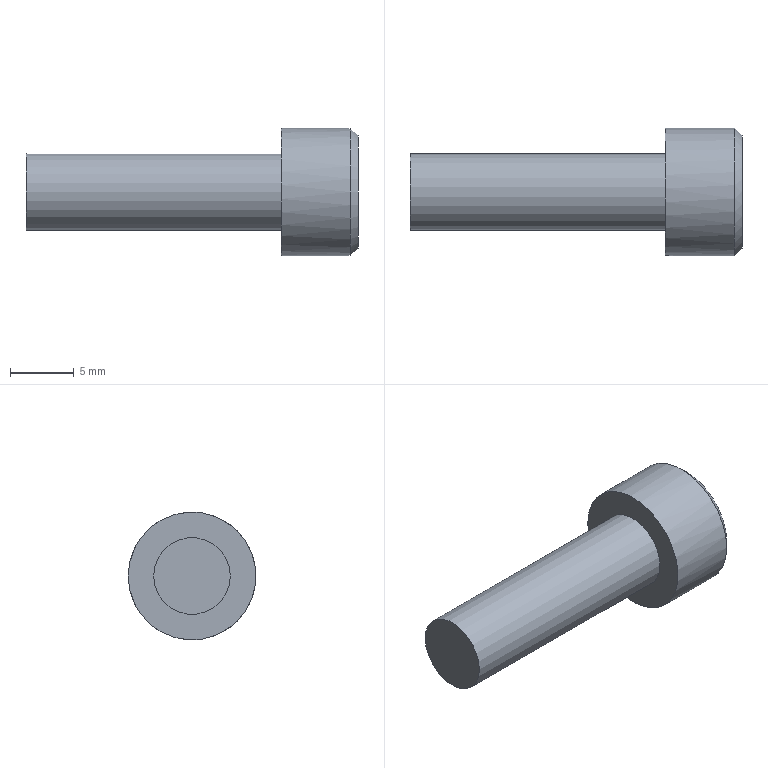Part | NX | features 5003_310_CB6-20 2 | 1 solid | 19 faces | box 26 x 10 x 10 mm | volume 956.513 mm3 | plane 15 | cylinder 2 | cone 2 | commonest cylinder face diameters 6 x1 10 x1
STEP:
#1=CARTESIAN_POINT('',(309.625,-201.4,-97.));
#2=VERTEX_POINT('',#1);
#3=CARTESIAN_POINT('',(309.625,-197.,-97.));
#4=DIRECTION('',(-1.,0.,0.));
#5=DIRECTION('',(0.,-1.,0.));
#6=AXIS2_PLACEMENT_3D('',#3,#4,#5);
#7=CIRCLE('',#6,4.4);
#8=EDGE_CURVE('',#2,#2,#7,.F.);
#9=ORIENTED_EDGE('',*,*,#8,.T.);
#10=EDGE_LOOP('',(#9));
#11=FACE_BOUND('',#10,.T.);
#12=CARTESIAN_POINT('',(309.625,-197.,-99.887));
#13=VERTEX_POINT('',#12);
#14=CARTESIAN_POINT('',(309.625,-194.5,-98.443));
#15=VERTEX_POINT('',#14);
#16=CARTESIAN_POINT('',(309.625,-197.,-99.887));
#17=DIRECTION('',(0.,0.866,0.5));
#18=VECTOR('',#17,1000.);
#19=LINE('',#16,#18);
#20=EDGE_CURVE('',#13,#15,#19,.T.);
#21=ORIENTED_EDGE('',*,*,#20,.F.);
#22=CARTESIAN_POINT('',(309.625,-199.5,-98.443));
#23=VERTEX_POINT('',#22);
#24=CARTESIAN_POINT('',(309.625,-199.5,-98.443));
#25=DIRECTION('',(0.,0.866,-0.5));
#26=VECTOR('',#25,1000.);
#27=LINE('',#24,#26);
#28=EDGE_CURVE('',#23,#13,#27,.T.);
#29=ORIENTED_EDGE('',*,*,#28,.F.);
#30=CARTESIAN_POINT('',(309.625,-199.5,-95.557));
#31=VERTEX_POINT('',#30);
#32=CARTESIAN_POINT('',(309.625,-199.5,-95.557));
#33=DIRECTION('',(0.,0.,-1.));
#34=VECTOR('',#33,1000.);
#35=LINE('',#32,#34);
#36=EDGE_CURVE('',#31,#23,#35,.T.);
#37=ORIENTED_EDGE('',*,*,#36,.F.);
#38=CARTESIAN_POINT('',(309.625,-197.,-94.113));
#39=VERTEX_POINT('',#38);
#40=CARTESIAN_POINT('',(309.625,-197.,-94.113));
#41=DIRECTION('',(0.,-0.866,-0.5));
#42=VECTOR('',#41,1000.);
#43=LINE('',#40,#42);
#44=EDGE_CURVE('',#39,#31,#43,.T.);
#45=ORIENTED_EDGE('',*,*,#44,.F.);
#46=CARTESIAN_POINT('',(309.625,-194.5,-95.557));
#47=VERTEX_POINT('',#46);
#48=CARTESIAN_POINT('',(309.625,-194.5,-95.557));
#49=DIRECTION('',(0.,-0.866,0.5));
#50=VECTOR('',#49,1000.);
#51=LINE('',#48,#50);
#52=EDGE_CURVE('',#47,#39,#51,.T.);
#53=ORIENTED_EDGE('',*,*,#52,.F.);
#54=CARTESIAN_POINT('',(309.625,-194.5,-98.443));
#55=DIRECTION('',(0.,0.,1.));
#56=VECTOR('',#55,1000.);
#57=LINE('',#54,#56);
#58=EDGE_CURVE('',#15,#47,#57,.T.);
#59=ORIENTED_EDGE('',*,*,#58,.F.);
#60=EDGE_LOOP('',(#21,#29,#37,#45,#53,#59));
#61=FACE_BOUND('',#60,.T.);
#62=CARTESIAN_POINT('',(309.625,-197.,-92.));
#63=DIRECTION('',(-1.,0.,0.));
#64=DIRECTION('',(0.,-1.,0.));
#65=AXIS2_PLACEMENT_3D('',#62,#63,#64);
#66=PLANE('',#65);
#67=ADVANCED_FACE('',(#11,#61),#66,.F.);
#68=CARTESIAN_POINT('',(283.625,-194.,-97.));
#69=VERTEX_POINT('',#68);
#70=CARTESIAN_POINT('',(283.625,-197.,-97.));
#71=DIRECTION('',(1.,0.,0.));
#72=DIRECTION('',(0.,1.,0.));
#73=AXIS2_PLACEMENT_3D('',#70,#71,#72);
#74=CIRCLE('',#73,3.);
#75=EDGE_CURVE('',#69,#69,#74,.T.);
#76=ORIENTED_EDGE('',*,*,#75,.F.);
#77=EDGE_LOOP('',(#76));
#78=FACE_BOUND('',#77,.T.);
#79=CARTESIAN_POINT('',(283.625,-197.,-97.));
#80=DIRECTION('',(1.,0.,0.));
#81=DIRECTION('',(0.,1.,0.));
#82=AXIS2_PLACEMENT_3D('',#79,#80,#81);
#83=PLANE('',#82);
#84=ADVANCED_FACE('',(#78),#83,.F.);
#85=CARTESIAN_POINT('',(303.625,-194.,-97.));
#86=VERTEX_POINT('',#85);
#87=CARTESIAN_POINT('',(303.625,-197.,-97.));
#88=DIRECTION('',(1.,0.,0.));
#89=DIRECTION('',(0.,1.,0.));
#90=AXIS2_PLACEMENT_3D('',#87,#88,#89);
#91=CIRCLE('',#90,3.);
#92=EDGE_CURVE('',#86,#86,#91,.T.);
#93=ORIENTED_EDGE('',*,*,#92,.F.);
#94=EDGE_LOOP('',(#93));
#95=FACE_BOUND('',#94,.T.);
#96=ORIENTED_EDGE('',*,*,#75,.T.);
#97=EDGE_LOOP('',(#96));
#98=FACE_BOUND('',#97,.T.);
#99=CARTESIAN_POINT('',(309.625,-197.,-97.));
#100=DIRECTION('',(1.,0.,0.));
#101=DIRECTION('',(0.,1.,0.));
#102=AXIS2_PLACEMENT_3D('',#99,#100,#101);
#103=CYLINDRICAL_SURFACE('',#102,3.);
#104=ADVANCED_FACE('',(#95,#98),#103,.T.);
#105=CARTESIAN_POINT('',(303.625,-192.,-97.));
#106=VERTEX_POINT('',#105);
#107=CARTESIAN_POINT('',(303.625,-197.,-97.));
#108=DIRECTION('',(1.,0.,0.));
#109=DIRECTION('',(0.,1.,0.));
#110=AXIS2_PLACEMENT_3D('',#107,#108,#109);
#111=CIRCLE('',#110,5.);
#112=EDGE_CURVE('',#106,#106,#111,.T.);
#113=ORIENTED_EDGE('',*,*,#112,.F.);
#114=EDGE_LOOP('',(#113));
#115=FACE_BOUND('',#114,.T.);
#116=ORIENTED_EDGE('',*,*,#92,.T.);
#117=EDGE_LOOP('',(#116));
#118=FACE_BOUND('',#117,.T.);
#119=CARTESIAN_POINT('',(303.625,-197.,-94.));
#120=DIRECTION('',(1.,0.,0.));
#121=DIRECTION('',(0.,1.,0.));
#122=AXIS2_PLACEMENT_3D('',#119,#120,#121);
#123=PLANE('',#122);
#124=ADVANCED_FACE('',(#115,#118),#123,.F.);
#125=CARTESIAN_POINT('',(309.025,-202.,-97.));
#126=VERTEX_POINT('',#125);
#127=CARTESIAN_POINT('',(309.025,-197.,-97.));
#128=DIRECTION('',(-1.,0.,0.));
#129=DIRECTION('',(0.,-1.,0.));
#130=AXIS2_PLACEMENT_3D('',#127,#128,#129);
#131=CIRCLE('',#130,5.);
#132=EDGE_CURVE('',#126,#126,#131,.T.);
#133=ORIENTED_EDGE('',*,*,#132,.T.);
#134=EDGE_LOOP('',(#133));
#135=FACE_BOUND('',#134,.T.);
#136=ORIENTED_EDGE('',*,*,#112,.T.);
#137=EDGE_LOOP('',(#136));
#138=FACE_BOUND('',#137,.T.);
#139=CARTESIAN_POINT('',(309.625,-197.,-97.));
#140=DIRECTION('',(1.,0.,0.));
#141=DIRECTION('',(0.,1.,0.));
#142=AXIS2_PLACEMENT_3D('',#139,#140,#141);
#143=CYLINDRICAL_SURFACE('',#142,5.);
#144=ADVANCED_FACE('',(#135,#138),#143,.T.);
#145=ORIENTED_EDGE('',*,*,#132,.F.);
#146=EDGE_LOOP('',(#145));
#147=FACE_BOUND('',#146,.T.);
#148=ORIENTED_EDGE('',*,*,#8,.F.);
#149=EDGE_LOOP('',(#148));
#150=FACE_BOUND('',#149,.T.);
#151=CARTESIAN_POINT('',(309.625,-197.,-97.));
#152=DIRECTION('',(-1.,0.,0.));
#153=DIRECTION('',(0.,-1.,0.));
#154=AXIS2_PLACEMENT_3D('',#151,#152,#153);
#155=CONICAL_SURFACE('',#154,4.4,0.7854);
#156=ADVANCED_FACE('',(#147,#150),#155,.T.);
#157=CARTESIAN_POINT('',(306.625,-199.5,-98.443));
#158=VERTEX_POINT('',#157);
#159=CARTESIAN_POINT('',(306.625,-198.25,-99.165));
#160=VERTEX_POINT('',#159);
#161=CARTESIAN_POINT('',(306.625,-199.5,-98.443));
#162=DIRECTION('',(0.,0.866,-0.5));
#163=VECTOR('',#162,1000.);
#164=LINE('',#161,#163);
#165=EDGE_CURVE('',#158,#160,#164,.T.);
#166=ORIENTED_EDGE('',*,*,#165,.F.);
#167=CARTESIAN_POINT('',(306.625,-199.5,-98.443));
#168=DIRECTION('',(1.,0.,0.));
#169=VECTOR('',#168,1000.);
#170=LINE('',#167,#169);
#171=EDGE_CURVE('',#158,#23,#170,.T.);
#172=ORIENTED_EDGE('',*,*,#171,.T.);
#173=ORIENTED_EDGE('',*,*,#28,.T.);
#174=CARTESIAN_POINT('',(306.625,-197.,-99.887));
#175=VERTEX_POINT('',#174);
#176=CARTESIAN_POINT('',(306.625,-197.,-99.887));
#177=DIRECTION('',(1.,0.,0.));
#178=VECTOR('',#177,1000.);
#179=LINE('',#176,#178);
#180=EDGE_CURVE('',#175,#13,#179,.T.);
#181=ORIENTED_EDGE('',*,*,#180,.F.);
#182=CARTESIAN_POINT('',(306.625,-199.5,-98.443));
#183=DIRECTION('',(0.,0.866,-0.5));
#184=VECTOR('',#183,1000.);
#185=LINE('',#182,#184);
#186=EDGE_CURVE('',#160,#175,#185,.T.);
#187=ORIENTED_EDGE('',*,*,#186,.F.);
#188=EDGE_LOOP('',(#166,#172,#173,#181,#187));
#189=FACE_BOUND('',#188,.T.);
#190=CARTESIAN_POINT('',(306.625,-199.5,-98.443));
#191=DIRECTION('',(0.,-0.5,-0.866));
#192=DIRECTION('',(0.,-0.866,0.5));
#193=AXIS2_PLACEMENT_3D('',#190,#191,#192);
#194=PLANE('',#193);
#195=ADVANCED_FACE('',(#189),#194,.F.);
#196=CARTESIAN_POINT('',(306.625,-199.5,-95.557));
#197=VERTEX_POINT('',#196);
#198=CARTESIAN_POINT('',(306.625,-199.5,-97.));
#199=VERTEX_POINT('',#198);
#200=CARTESIAN_POINT('',(306.625,-199.5,-95.557));
#201=DIRECTION('',(0.,0.,-1.));
#202=VECTOR('',#201,1000.);
#203=LINE('',#200,#202);
#204=EDGE_CURVE('',#197,#199,#203,.T.);
#205=ORIENTED_EDGE('',*,*,#204,.F.);
#206=CARTESIAN_POINT('',(306.625,-199.5,-95.557));
#207=DIRECTION('',(1.,0.,0.));
#208=VECTOR('',#207,1000.);
#209=LINE('',#206,#208);
#210=EDGE_CURVE('',#197,#31,#209,.T.);
#211=ORIENTED_EDGE('',*,*,#210,.T.);
#212=ORIENTED_EDGE('',*,*,#36,.T.);
#213=ORIENTED_EDGE('',*,*,#171,.F.);
#214=CARTESIAN_POINT('',(306.625,-199.5,-95.557));
#215=DIRECTION('',(0.,0.,-1.));
#216=VECTOR('',#215,1000.);
#217=LINE('',#214,#216);
#218=EDGE_CURVE('',#199,#158,#217,.T.);
#219=ORIENTED_EDGE('',*,*,#218,.F.);
#220=EDGE_LOOP('',(#205,#211,#212,#213,#219));
#221=FACE_BOUND('',#220,.T.);
#222=CARTESIAN_POINT('',(306.625,-199.5,-95.557));
#223=DIRECTION('',(0.,-1.,0.));
#224=DIRECTION('',(0.,0.,1.));
#225=AXIS2_PLACEMENT_3D('',#222,#223,#224);
#226=PLANE('',#225);
#227=ADVANCED_FACE('',(#221),#226,.F.);
#228=CARTESIAN_POINT('',(306.625,-197.,-94.113));
#229=VERTEX_POINT('',#228);
#230=CARTESIAN_POINT('',(306.625,-198.25,-94.835));
#231=VERTEX_POINT('',#230);
#232=CARTESIAN_POINT('',(306.625,-197.,-94.113));
#233=DIRECTION('',(0.,-0.866,-0.5));
#234=VECTOR('',#233,1000.);
#235=LINE('',#232,#234);
#236=EDGE_CURVE('',#229,#231,#235,.T.);
#237=ORIENTED_EDGE('',*,*,#236,.F.);
#238=CARTESIAN_POINT('',(306.625,-197.,-94.113));
#239=DIRECTION('',(1.,0.,0.));
#240=VECTOR('',#239,1000.);
#241=LINE('',#238,#240);
#242=EDGE_CURVE('',#229,#39,#241,.T.);
#243=ORIENTED_EDGE('',*,*,#242,.T.);
#244=ORIENTED_EDGE('',*,*,#44,.T.);
#245=ORIENTED_EDGE('',*,*,#210,.F.);
#246=CARTESIAN_POINT('',(306.625,-197.,-94.113));
#247=DIRECTION('',(0.,-0.866,-0.5));
#248=VECTOR('',#247,1000.);
#249=LINE('',#246,#248);
#250=EDGE_CURVE('',#231,#197,#249,.T.);
#251=ORIENTED_EDGE('',*,*,#250,.F.);
#252=EDGE_LOOP('',(#237,#243,#244,#245,#251));
#253=FACE_BOUND('',#252,.T.);
#254=CARTESIAN_POINT('',(306.625,-197.,-94.113));
#255=DIRECTION('',(0.,-0.5,0.866));
#256=DIRECTION('',(0.,0.866,0.5));
#257=AXIS2_PLACEMENT_3D('',#254,#255,#256);
#258=PLANE('',#257);
#259=ADVANCED_FACE('',(#253),#258,.F.);
#260=CARTESIAN_POINT('',(306.625,-194.5,-95.557));
#261=VERTEX_POINT('',#260);
#262=CARTESIAN_POINT('',(306.625,-195.75,-94.835));
#263=VERTEX_POINT('',#262);
#264=CARTESIAN_POINT('',(306.625,-194.5,-95.557));
#265=DIRECTION('',(0.,-0.866,0.5));
#266=VECTOR('',#265,1000.);
#267=LINE('',#264,#266);
#268=EDGE_CURVE('',#261,#263,#267,.T.);
#269=ORIENTED_EDGE('',*,*,#268,.F.);
#270=CARTESIAN_POINT('',(306.625,-194.5,-95.557));
#271=DIRECTION('',(1.,0.,0.));
#272=VECTOR('',#271,1000.);
#273=LINE('',#270,#272);
#274=EDGE_CURVE('',#261,#47,#273,.T.);
#275=ORIENTED_EDGE('',*,*,#274,.T.);
#276=ORIENTED_EDGE('',*,*,#52,.T.);
#277=ORIENTED_EDGE('',*,*,#242,.F.);
#278=CARTESIAN_POINT('',(306.625,-194.5,-95.557));
#279=DIRECTION('',(0.,-0.866,0.5));
#280=VECTOR('',#279,1000.);
#281=LINE('',#278,#280);
#282=EDGE_CURVE('',#263,#229,#281,.T.);
#283=ORIENTED_EDGE('',*,*,#282,.F.);
#284=EDGE_LOOP('',(#269,#275,#276,#277,#283));
#285=FACE_BOUND('',#284,.T.);
#286=CARTESIAN_POINT('',(306.625,-194.5,-95.557));
#287=DIRECTION('',(0.,0.5,0.866));
#288=DIRECTION('',(0.,0.866,-0.5));
#289=AXIS2_PLACEMENT_3D('',#286,#287,#288);
#290=PLANE('',#289);
#291=ADVANCED_FACE('',(#285),#290,.F.);
#292=CARTESIAN_POINT('',(306.625,-194.5,-98.443));
#293=VERTEX_POINT('',#292);
#294=CARTESIAN_POINT('',(306.625,-194.5,-97.));
#295=VERTEX_POINT('',#294);
#296=CARTESIAN_POINT('',(306.625,-194.5,-98.443));
#297=DIRECTION('',(0.,0.,1.));
#298=VECTOR('',#297,1000.);
#299=LINE('',#296,#298);
#300=EDGE_CURVE('',#293,#295,#299,.T.);
#301=ORIENTED_EDGE('',*,*,#300,.F.);
#302=CARTESIAN_POINT('',(306.625,-194.5,-98.443));
#303=DIRECTION('',(1.,0.,0.));
#304=VECTOR('',#303,1000.);
#305=LINE('',#302,#304);
#306=EDGE_CURVE('',#293,#15,#305,.T.);
#307=ORIENTED_EDGE('',*,*,#306,.T.);
#308=ORIENTED_EDGE('',*,*,#58,.T.);
#309=ORIENTED_EDGE('',*,*,#274,.F.);
#310=CARTESIAN_POINT('',(306.625,-194.5,-98.443));
#311=DIRECTION('',(0.,0.,1.));
#312=VECTOR('',#311,1000.);
#313=LINE('',#310,#312);
#314=EDGE_CURVE('',#295,#261,#313,.T.);
#315=ORIENTED_EDGE('',*,*,#314,.F.);
#316=EDGE_LOOP('',(#301,#307,#308,#309,#315));
#317=FACE_BOUND('',#316,.T.);
#318=CARTESIAN_POINT('',(306.625,-194.5,-98.443));
#319=DIRECTION('',(0.,1.,0.));
#320=DIRECTION('',(-1.,0.,0.));
#321=AXIS2_PLACEMENT_3D('',#318,#319,#320);
#322=PLANE('',#321);
#323=ADVANCED_FACE('',(#317),#322,.F.);
#324=CARTESIAN_POINT('',(306.625,-195.75,-99.165));
#325=VERTEX_POINT('',#324);
#326=CARTESIAN_POINT('',(306.625,-197.,-99.887));
#327=DIRECTION('',(0.,0.866,0.5));
#328=VECTOR('',#327,1000.);
#329=LINE('',#326,#328);
#330=EDGE_CURVE('',#175,#325,#329,.T.);
#331=ORIENTED_EDGE('',*,*,#330,.F.);
#332=ORIENTED_EDGE('',*,*,#180,.T.);
#333=ORIENTED_EDGE('',*,*,#20,.T.);
#334=ORIENTED_EDGE('',*,*,#306,.F.);
#335=CARTESIAN_POINT('',(306.625,-197.,-99.887));
#336=DIRECTION('',(0.,0.866,0.5));
#337=VECTOR('',#336,1000.);
#338=LINE('',#335,#337);
#339=EDGE_CURVE('',#325,#293,#338,.T.);
#340=ORIENTED_EDGE('',*,*,#339,.F.);
#341=EDGE_LOOP('',(#331,#332,#333,#334,#340));
#342=FACE_BOUND('',#341,.T.);
#343=CARTESIAN_POINT('',(306.625,-197.,-99.887));
#344=DIRECTION('',(0.,0.5,-0.866));
#345=DIRECTION('',(0.,-0.866,-0.5));
#346=AXIS2_PLACEMENT_3D('',#343,#344,#345);
#347=PLANE('',#346);
#348=ADVANCED_FACE('',(#342),#347,.F.);
#349=ORIENTED_EDGE('',*,*,#314,.T.);
#350=ORIENTED_EDGE('',*,*,#268,.T.);
#351=CARTESIAN_POINT('',(306.625,-197.,-97.));
#352=DIRECTION('',(1.,0.,0.));
#353=DIRECTION('',(0.,0.,-1.));
#354=AXIS2_PLACEMENT_3D('',#351,#352,#353);
#355=CIRCLE('',#354,2.5);
#356=EDGE_CURVE('',#295,#263,#355,.T.);
#357=ORIENTED_EDGE('',*,*,#356,.F.);
#358=EDGE_LOOP('',(#349,#350,#357));
#359=FACE_BOUND('',#358,.T.);
#360=CARTESIAN_POINT('',(306.625,-197.,-97.));
#361=DIRECTION('',(1.,0.,0.));
#362=DIRECTION('',(0.,1.,0.));
#363=AXIS2_PLACEMENT_3D('',#360,#361,#362);
#364=PLANE('',#363);
#365=ADVANCED_FACE('',(#359),#364,.T.);
#366=ORIENTED_EDGE('',*,*,#282,.T.);
#367=ORIENTED_EDGE('',*,*,#236,.T.);
#368=CARTESIAN_POINT('',(306.625,-197.,-97.));
#369=DIRECTION('',(1.,0.,0.));
#370=DIRECTION('',(0.,0.,-1.));
#371=AXIS2_PLACEMENT_3D('',#368,#369,#370);
#372=CIRCLE('',#371,2.5);
#373=EDGE_CURVE('',#263,#231,#372,.T.);
#374=ORIENTED_EDGE('',*,*,#373,.F.);
#375=EDGE_LOOP('',(#366,#367,#374));
#376=FACE_BOUND('',#375,.T.);
#377=CARTESIAN_POINT('',(306.625,-197.,-97.));
#378=DIRECTION('',(1.,0.,0.));
#379=DIRECTION('',(0.,1.,0.));
#380=AXIS2_PLACEMENT_3D('',#377,#378,#379);
#381=PLANE('',#380);
#382=ADVANCED_FACE('',(#376),#381,.T.);
#383=ORIENTED_EDGE('',*,*,#250,.T.);
#384=ORIENTED_EDGE('',*,*,#204,.T.);
#385=CARTESIAN_POINT('',(306.625,-197.,-97.));
#386=DIRECTION('',(1.,0.,0.));
#387=DIRECTION('',(0.,0.,-1.));
#388=AXIS2_PLACEMENT_3D('',#385,#386,#387);
#389=CIRCLE('',#388,2.5);
#390=EDGE_CURVE('',#231,#199,#389,.T.);
#391=ORIENTED_EDGE('',*,*,#390,.F.);
#392=EDGE_LOOP('',(#383,#384,#391));
#393=FACE_BOUND('',#392,.T.);
#394=CARTESIAN_POINT('',(306.625,-197.,-97.));
#395=DIRECTION('',(1.,0.,0.));
#396=DIRECTION('',(0.,1.,0.));
#397=AXIS2_PLACEMENT_3D('',#394,#395,#396);
#398=PLANE('',#397);
#399=ADVANCED_FACE('',(#393),#398,.T.);
#400=ORIENTED_EDGE('',*,*,#218,.T.);
#401=ORIENTED_EDGE('',*,*,#165,.T.);
#402=CARTESIAN_POINT('',(306.625,-197.,-97.));
#403=DIRECTION('',(1.,0.,0.));
#404=DIRECTION('',(0.,0.,-1.));
#405=AXIS2_PLACEMENT_3D('',#402,#403,#404);
#406=CIRCLE('',#405,2.5);
#407=EDGE_CURVE('',#199,#160,#406,.T.);
#408=ORIENTED_EDGE('',*,*,#407,.F.);
#409=EDGE_LOOP('',(#400,#401,#408));
#410=FACE_BOUND('',#409,.T.);
#411=CARTESIAN_POINT('',(306.625,-197.,-97.));
#412=DIRECTION('',(1.,0.,0.));
#413=DIRECTION('',(0.,1.,0.));
#414=AXIS2_PLACEMENT_3D('',#411,#412,#413);
#415=PLANE('',#414);
#416=ADVANCED_FACE('',(#410),#415,.T.);
#417=ORIENTED_EDGE('',*,*,#186,.T.);
#418=ORIENTED_EDGE('',*,*,#330,.T.);
#419=CARTESIAN_POINT('',(306.625,-197.,-97.));
#420=DIRECTION('',(1.,0.,0.));
#421=DIRECTION('',(0.,0.,-1.));
#422=AXIS2_PLACEMENT_3D('',#419,#420,#421);
#423=CIRCLE('',#422,2.5);
#424=EDGE_CURVE('',#160,#325,#423,.T.);
#425=ORIENTED_EDGE('',*,*,#424,.F.);
#426=EDGE_LOOP('',(#417,#418,#425));
#427=FACE_BOUND('',#426,.T.);
#428=CARTESIAN_POINT('',(306.625,-197.,-97.));
#429=DIRECTION('',(1.,0.,0.));
#430=DIRECTION('',(0.,1.,0.));
#431=AXIS2_PLACEMENT_3D('',#428,#429,#430);
#432=PLANE('',#431);
#433=ADVANCED_FACE('',(#427),#432,.T.);
#434=ORIENTED_EDGE('',*,*,#339,.T.);
#435=ORIENTED_EDGE('',*,*,#300,.T.);
#436=CARTESIAN_POINT('',(306.625,-197.,-97.));
#437=DIRECTION('',(1.,0.,0.));
#438=DIRECTION('',(0.,0.,-1.));
#439=AXIS2_PLACEMENT_3D('',#436,#437,#438);
#440=CIRCLE('',#439,2.5);
#441=EDGE_CURVE('',#325,#295,#440,.T.);
#442=ORIENTED_EDGE('',*,*,#441,.F.);
#443=EDGE_LOOP('',(#434,#435,#442));
#444=FACE_BOUND('',#443,.T.);
#445=CARTESIAN_POINT('',(306.625,-197.,-97.));
#446=DIRECTION('',(1.,0.,0.));
#447=DIRECTION('',(0.,1.,0.));
#448=AXIS2_PLACEMENT_3D('',#445,#446,#447);
#449=PLANE('',#448);
#450=ADVANCED_FACE('',(#444),#449,.T.);
#451=ORIENTED_EDGE('',*,*,#441,.T.);
#452=ORIENTED_EDGE('',*,*,#356,.T.);
#453=ORIENTED_EDGE('',*,*,#373,.T.);
#454=ORIENTED_EDGE('',*,*,#390,.T.);
#455=ORIENTED_EDGE('',*,*,#407,.T.);
#456=ORIENTED_EDGE('',*,*,#424,.T.);
#457=EDGE_LOOP('',(#451,#452,#453,#454,#455,#456));
#458=FACE_BOUND('',#457,.T.);
#459=CARTESIAN_POINT('',(305.123,-197.,-97.));
#460=VERTEX_POINT('',#459);
#461=VERTEX_LOOP('',#460);
#462=FACE_BOUND('',#461,.T.);
#463=CARTESIAN_POINT('',(305.123,-197.,-97.));
#464=DIRECTION('',(1.,0.,0.));
#465=DIRECTION('',(0.,0.,-1.));
#466=AXIS2_PLACEMENT_3D('',#463,#464,#465);
#467=CONICAL_SURFACE('',#466,0.,1.03);
#468=ADVANCED_FACE('',(#458,#462),#467,.F.);
#469=CLOSED_SHELL('',(#67,#84,#104,#124,#144,#156,#195,#227,#259,#291,#323,#348,#365,#382,#399,#416,#433,#450,#468));
#470=MANIFOLD_SOLID_BREP('',#469);
#471=(LENGTH_UNIT()NAMED_UNIT(*)SI_UNIT(.MILLI.,.METRE.));
#472=UNCERTAINTY_MEASURE_WITH_UNIT(LENGTH_MEASURE(0.00001),#471,'','');
#473=(NAMED_UNIT(*)PLANE_ANGLE_UNIT()SI_UNIT($,.RADIAN.));
#474=(NAMED_UNIT(*)SI_UNIT($,.STERADIAN.)SOLID_ANGLE_UNIT());
#475=(GEOMETRIC_REPRESENTATION_CONTEXT(3)GLOBAL_UNCERTAINTY_ASSIGNED_CONTEXT((#472))GLOBAL_UNIT_ASSIGNED_CONTEXT((#471,#473,#474))REPRESENTATION_CONTEXT('',''));
#476=ADVANCED_BREP_SHAPE_REPRESENTATION('',(#470),#475);